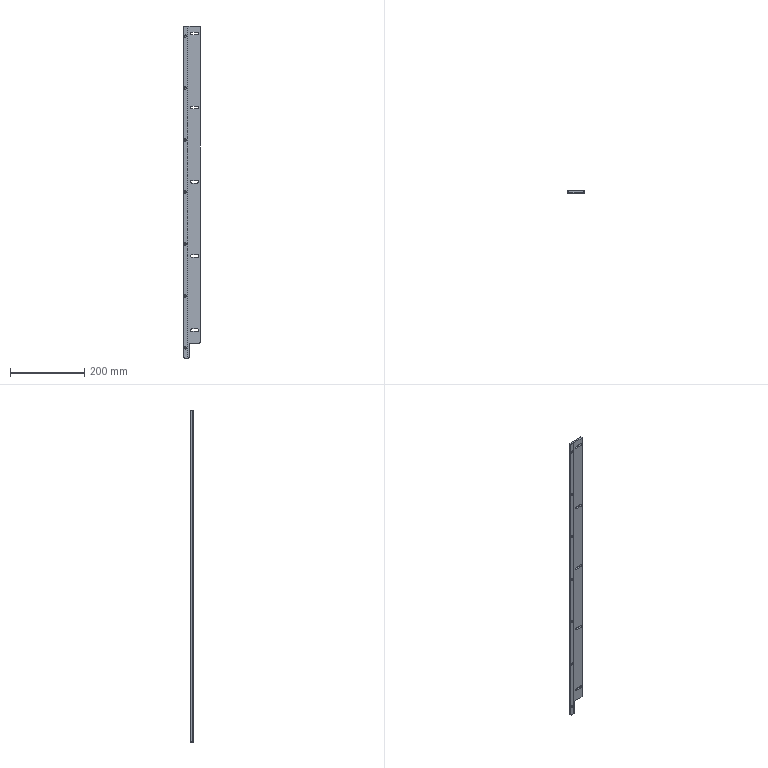Part | STEP file | BZJ-BZMM-JDKTBDYY Product限位Plate四 | 1 solid | 63 faces | box 44 x 6 x 895 mm | volume 219689 mm3 | cylinder 29 | plane 20 | cone 14 | commonest cylinder face diameters 2.5 x14 6.6 x10 4 x5